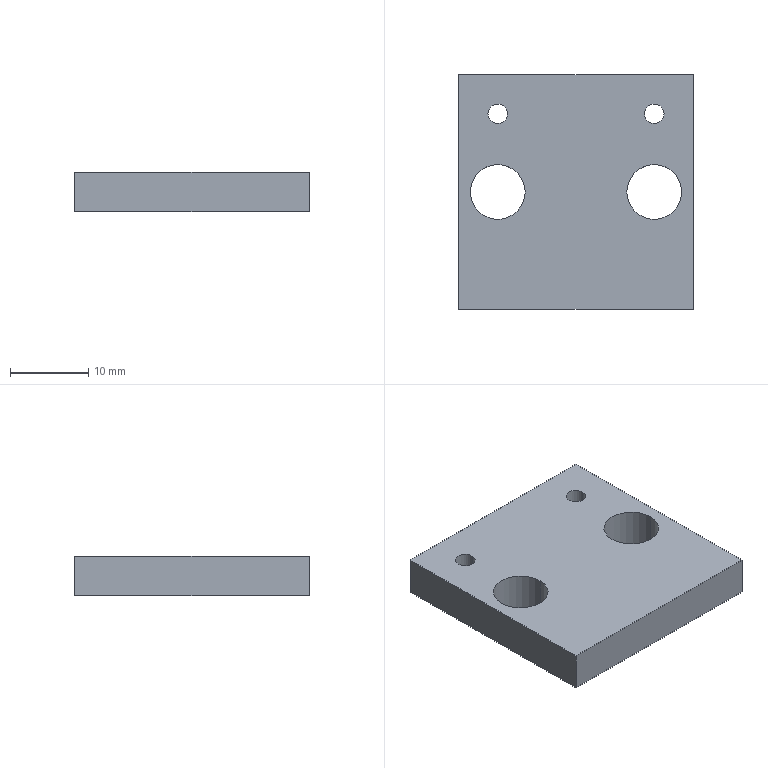Part | SolidWorks | features Extrusion 1, HoleWzd 1 | 1 solid | 14 faces | box 30 x 30 x 5 mm | volume 4066 mm3 | cylinder 8 | plane 6 | commonest cylinder face diameters 2.5 x4 7 x4
STEP:
#1=CARTESIAN_POINT('',(6.5,0.,0.));
#2=VERTEX_POINT('',#1);
#3=CARTESIAN_POINT('',(13.5,0.,0.));
#4=VERTEX_POINT('',#3);
#5=CARTESIAN_POINT('',(10.,0.,0.));
#6=DIRECTION('',(0.,0.,1.));
#7=DIRECTION('',(1.,0.,0.));
#8=AXIS2_PLACEMENT_3D('',#5,#6,#7);
#9=CIRCLE('',#8,3.5);
#10=EDGE_CURVE('',#2,#4,#9,.T.);
#11=ORIENTED_EDGE('',*,*,#10,.F.);
#12=CARTESIAN_POINT('',(6.5,0.,5.));
#13=VERTEX_POINT('',#12);
#14=CARTESIAN_POINT('',(6.5,0.,5.));
#15=DIRECTION('',(0.,0.,1.));
#16=VECTOR('',#15,1000.);
#17=LINE('',#14,#16);
#18=EDGE_CURVE('',#2,#13,#17,.T.);
#19=ORIENTED_EDGE('',*,*,#18,.T.);
#20=CARTESIAN_POINT('',(13.5,0.,5.));
#21=VERTEX_POINT('',#20);
#22=CARTESIAN_POINT('',(10.,0.,5.));
#23=DIRECTION('',(0.,0.,1.));
#24=DIRECTION('',(1.,0.,0.));
#25=AXIS2_PLACEMENT_3D('',#22,#23,#24);
#26=CIRCLE('',#25,3.5);
#27=EDGE_CURVE('',#13,#21,#26,.T.);
#28=ORIENTED_EDGE('',*,*,#27,.T.);
#29=CARTESIAN_POINT('',(13.5,0.,5.));
#30=DIRECTION('',(0.,0.,1.));
#31=VECTOR('',#30,1000.);
#32=LINE('',#29,#31);
#33=EDGE_CURVE('',#4,#21,#32,.T.);
#34=ORIENTED_EDGE('',*,*,#33,.F.);
#35=EDGE_LOOP('',(#11,#19,#28,#34));
#36=FACE_OUTER_BOUND('',#35,.T.);
#37=CARTESIAN_POINT('',(10.,0.,5.));
#38=DIRECTION('',(0.,0.,1.));
#39=DIRECTION('',(1.,0.,0.));
#40=AXIS2_PLACEMENT_3D('',#37,#38,#39);
#41=CYLINDRICAL_SURFACE('',#40,3.5);
#42=ADVANCED_FACE('',(#36),#41,.F.);
#43=CARTESIAN_POINT('',(-13.5,0.,0.));
#44=VERTEX_POINT('',#43);
#45=CARTESIAN_POINT('',(-6.5,0.,0.));
#46=VERTEX_POINT('',#45);
#47=CARTESIAN_POINT('',(-10.,0.,0.));
#48=DIRECTION('',(0.,0.,1.));
#49=DIRECTION('',(1.,0.,0.));
#50=AXIS2_PLACEMENT_3D('',#47,#48,#49);
#51=CIRCLE('',#50,3.5);
#52=EDGE_CURVE('',#44,#46,#51,.T.);
#53=ORIENTED_EDGE('',*,*,#52,.F.);
#54=CARTESIAN_POINT('',(-13.5,0.,5.));
#55=VERTEX_POINT('',#54);
#56=CARTESIAN_POINT('',(-13.5,0.,5.));
#57=DIRECTION('',(0.,0.,1.));
#58=VECTOR('',#57,1000.);
#59=LINE('',#56,#58);
#60=EDGE_CURVE('',#44,#55,#59,.T.);
#61=ORIENTED_EDGE('',*,*,#60,.T.);
#62=CARTESIAN_POINT('',(-6.5,0.,5.));
#63=VERTEX_POINT('',#62);
#64=CARTESIAN_POINT('',(-10.,0.,5.));
#65=DIRECTION('',(0.,0.,1.));
#66=DIRECTION('',(1.,0.,0.));
#67=AXIS2_PLACEMENT_3D('',#64,#65,#66);
#68=CIRCLE('',#67,3.5);
#69=EDGE_CURVE('',#55,#63,#68,.T.);
#70=ORIENTED_EDGE('',*,*,#69,.T.);
#71=CARTESIAN_POINT('',(-6.5,0.,5.));
#72=DIRECTION('',(0.,0.,1.));
#73=VECTOR('',#72,1000.);
#74=LINE('',#71,#73);
#75=EDGE_CURVE('',#46,#63,#74,.T.);
#76=ORIENTED_EDGE('',*,*,#75,.F.);
#77=EDGE_LOOP('',(#53,#61,#70,#76));
#78=FACE_OUTER_BOUND('',#77,.T.);
#79=CARTESIAN_POINT('',(-10.,0.,5.));
#80=DIRECTION('',(0.,0.,1.));
#81=DIRECTION('',(1.,0.,0.));
#82=AXIS2_PLACEMENT_3D('',#79,#80,#81);
#83=CYLINDRICAL_SURFACE('',#82,3.5);
#84=ADVANCED_FACE('',(#78),#83,.F.);
#85=CARTESIAN_POINT('',(8.75,10.,0.));
#86=VERTEX_POINT('',#85);
#87=CARTESIAN_POINT('',(11.25,10.,0.));
#88=VERTEX_POINT('',#87);
#89=CARTESIAN_POINT('',(10.,10.,0.));
#90=DIRECTION('',(0.,0.,1.));
#91=DIRECTION('',(-1.,0.,0.));
#92=AXIS2_PLACEMENT_3D('',#89,#90,#91);
#93=CIRCLE('',#92,1.25);
#94=EDGE_CURVE('',#86,#88,#93,.T.);
#95=ORIENTED_EDGE('',*,*,#94,.F.);
#96=CARTESIAN_POINT('',(8.75,10.,5.));
#97=VERTEX_POINT('',#96);
#98=CARTESIAN_POINT('',(8.75,10.,0.));
#99=DIRECTION('',(0.,0.,1.));
#100=VECTOR('',#99,1000.);
#101=LINE('',#98,#100);
#102=EDGE_CURVE('',#86,#97,#101,.T.);
#103=ORIENTED_EDGE('',*,*,#102,.T.);
#104=CARTESIAN_POINT('',(11.25,10.,5.));
#105=VERTEX_POINT('',#104);
#106=CARTESIAN_POINT('',(10.,10.,5.));
#107=DIRECTION('',(0.,0.,1.));
#108=DIRECTION('',(-1.,0.,0.));
#109=AXIS2_PLACEMENT_3D('',#106,#107,#108);
#110=CIRCLE('',#109,1.25);
#111=EDGE_CURVE('',#97,#105,#110,.T.);
#112=ORIENTED_EDGE('',*,*,#111,.T.);
#113=CARTESIAN_POINT('',(11.25,10.,0.));
#114=DIRECTION('',(0.,0.,1.));
#115=VECTOR('',#114,1000.);
#116=LINE('',#113,#115);
#117=EDGE_CURVE('',#88,#105,#116,.T.);
#118=ORIENTED_EDGE('',*,*,#117,.F.);
#119=EDGE_LOOP('',(#95,#103,#112,#118));
#120=FACE_OUTER_BOUND('',#119,.T.);
#121=CARTESIAN_POINT('',(10.,10.,0.));
#122=DIRECTION('',(0.,0.,1.));
#123=DIRECTION('',(1.,0.,0.));
#124=AXIS2_PLACEMENT_3D('',#121,#122,#123);
#125=CYLINDRICAL_SURFACE('',#124,1.25);
#126=ADVANCED_FACE('',(#120),#125,.F.);
#127=CARTESIAN_POINT('',(-11.25,10.,0.));
#128=VERTEX_POINT('',#127);
#129=CARTESIAN_POINT('',(-8.75,10.,0.));
#130=VERTEX_POINT('',#129);
#131=CARTESIAN_POINT('',(-10.,10.,0.));
#132=DIRECTION('',(0.,0.,1.));
#133=DIRECTION('',(-1.,0.,0.));
#134=AXIS2_PLACEMENT_3D('',#131,#132,#133);
#135=CIRCLE('',#134,1.25);
#136=EDGE_CURVE('',#128,#130,#135,.T.);
#137=ORIENTED_EDGE('',*,*,#136,.F.);
#138=CARTESIAN_POINT('',(-11.25,10.,5.));
#139=VERTEX_POINT('',#138);
#140=CARTESIAN_POINT('',(-11.25,10.,0.));
#141=DIRECTION('',(0.,0.,1.));
#142=VECTOR('',#141,1000.);
#143=LINE('',#140,#142);
#144=EDGE_CURVE('',#128,#139,#143,.T.);
#145=ORIENTED_EDGE('',*,*,#144,.T.);
#146=CARTESIAN_POINT('',(-8.75,10.,5.));
#147=VERTEX_POINT('',#146);
#148=CARTESIAN_POINT('',(-10.,10.,5.));
#149=DIRECTION('',(0.,0.,1.));
#150=DIRECTION('',(-1.,0.,0.));
#151=AXIS2_PLACEMENT_3D('',#148,#149,#150);
#152=CIRCLE('',#151,1.25);
#153=EDGE_CURVE('',#139,#147,#152,.T.);
#154=ORIENTED_EDGE('',*,*,#153,.T.);
#155=CARTESIAN_POINT('',(-8.75,10.,0.));
#156=DIRECTION('',(0.,0.,1.));
#157=VECTOR('',#156,1000.);
#158=LINE('',#155,#157);
#159=EDGE_CURVE('',#130,#147,#158,.T.);
#160=ORIENTED_EDGE('',*,*,#159,.F.);
#161=EDGE_LOOP('',(#137,#145,#154,#160));
#162=FACE_OUTER_BOUND('',#161,.T.);
#163=CARTESIAN_POINT('',(-10.,10.,0.));
#164=DIRECTION('',(0.,0.,1.));
#165=DIRECTION('',(1.,0.,0.));
#166=AXIS2_PLACEMENT_3D('',#163,#164,#165);
#167=CYLINDRICAL_SURFACE('',#166,1.25);
#168=ADVANCED_FACE('',(#162),#167,.F.);
#169=CARTESIAN_POINT('',(-15.,15.,5.));
#170=VERTEX_POINT('',#169);
#171=CARTESIAN_POINT('',(-15.,-15.,5.));
#172=VERTEX_POINT('',#171);
#173=CARTESIAN_POINT('',(-15.,15.,5.));
#174=DIRECTION('',(0.,-1.,0.));
#175=VECTOR('',#174,1000.);
#176=LINE('',#173,#175);
#177=EDGE_CURVE('',#170,#172,#176,.T.);
#178=ORIENTED_EDGE('',*,*,#177,.F.);
#179=CARTESIAN_POINT('',(-15.,15.,0.));
#180=VERTEX_POINT('',#179);
#181=CARTESIAN_POINT('',(-15.,15.,0.));
#182=DIRECTION('',(0.,0.,1.));
#183=VECTOR('',#182,1000.);
#184=LINE('',#181,#183);
#185=EDGE_CURVE('',#180,#170,#184,.T.);
#186=ORIENTED_EDGE('',*,*,#185,.F.);
#187=CARTESIAN_POINT('',(-15.,-15.,0.));
#188=VERTEX_POINT('',#187);
#189=CARTESIAN_POINT('',(-15.,15.,0.));
#190=DIRECTION('',(0.,-1.,0.));
#191=VECTOR('',#190,1000.);
#192=LINE('',#189,#191);
#193=EDGE_CURVE('',#180,#188,#192,.T.);
#194=ORIENTED_EDGE('',*,*,#193,.T.);
#195=CARTESIAN_POINT('',(-15.,-15.,0.));
#196=DIRECTION('',(0.,0.,1.));
#197=VECTOR('',#196,1000.);
#198=LINE('',#195,#197);
#199=EDGE_CURVE('',#188,#172,#198,.T.);
#200=ORIENTED_EDGE('',*,*,#199,.T.);
#201=EDGE_LOOP('',(#178,#186,#194,#200));
#202=FACE_OUTER_BOUND('',#201,.T.);
#203=CARTESIAN_POINT('',(-15.,15.,0.));
#204=DIRECTION('',(-1.,0.,0.));
#205=DIRECTION('',(0.,-1.,0.));
#206=AXIS2_PLACEMENT_3D('',#203,#204,#205);
#207=PLANE('',#206);
#208=ADVANCED_FACE('',(#202),#207,.T.);
#209=CARTESIAN_POINT('',(15.,15.,5.));
#210=VERTEX_POINT('',#209);
#211=CARTESIAN_POINT('',(15.,15.,5.));
#212=DIRECTION('',(-1.,0.,0.));
#213=VECTOR('',#212,1000.);
#214=LINE('',#211,#213);
#215=EDGE_CURVE('',#210,#170,#214,.T.);
#216=ORIENTED_EDGE('',*,*,#215,.F.);
#217=CARTESIAN_POINT('',(15.,15.,0.));
#218=VERTEX_POINT('',#217);
#219=CARTESIAN_POINT('',(15.,15.,0.));
#220=DIRECTION('',(0.,0.,1.));
#221=VECTOR('',#220,1000.);
#222=LINE('',#219,#221);
#223=EDGE_CURVE('',#218,#210,#222,.T.);
#224=ORIENTED_EDGE('',*,*,#223,.F.);
#225=CARTESIAN_POINT('',(15.,15.,0.));
#226=DIRECTION('',(-1.,0.,0.));
#227=VECTOR('',#226,1000.);
#228=LINE('',#225,#227);
#229=EDGE_CURVE('',#218,#180,#228,.T.);
#230=ORIENTED_EDGE('',*,*,#229,.T.);
#231=ORIENTED_EDGE('',*,*,#185,.T.);
#232=EDGE_LOOP('',(#216,#224,#230,#231));
#233=FACE_OUTER_BOUND('',#232,.T.);
#234=CARTESIAN_POINT('',(15.,15.,0.));
#235=DIRECTION('',(0.,1.,0.));
#236=DIRECTION('',(-1.,0.,0.));
#237=AXIS2_PLACEMENT_3D('',#234,#235,#236);
#238=PLANE('',#237);
#239=ADVANCED_FACE('',(#233),#238,.T.);
#240=CARTESIAN_POINT('',(15.,-15.,5.));
#241=VERTEX_POINT('',#240);
#242=CARTESIAN_POINT('',(15.,-15.,5.));
#243=DIRECTION('',(0.,1.,0.));
#244=VECTOR('',#243,1000.);
#245=LINE('',#242,#244);
#246=EDGE_CURVE('',#241,#210,#245,.T.);
#247=ORIENTED_EDGE('',*,*,#246,.F.);
#248=CARTESIAN_POINT('',(15.,-15.,0.));
#249=VERTEX_POINT('',#248);
#250=CARTESIAN_POINT('',(15.,-15.,0.));
#251=DIRECTION('',(0.,0.,1.));
#252=VECTOR('',#251,1000.);
#253=LINE('',#250,#252);
#254=EDGE_CURVE('',#249,#241,#253,.T.);
#255=ORIENTED_EDGE('',*,*,#254,.F.);
#256=CARTESIAN_POINT('',(15.,-15.,0.));
#257=DIRECTION('',(0.,1.,0.));
#258=VECTOR('',#257,1000.);
#259=LINE('',#256,#258);
#260=EDGE_CURVE('',#249,#218,#259,.T.);
#261=ORIENTED_EDGE('',*,*,#260,.T.);
#262=ORIENTED_EDGE('',*,*,#223,.T.);
#263=EDGE_LOOP('',(#247,#255,#261,#262));
#264=FACE_OUTER_BOUND('',#263,.T.);
#265=CARTESIAN_POINT('',(15.,-15.,0.));
#266=DIRECTION('',(1.,0.,0.));
#267=DIRECTION('',(0.,1.,0.));
#268=AXIS2_PLACEMENT_3D('',#265,#266,#267);
#269=PLANE('',#268);
#270=ADVANCED_FACE('',(#264),#269,.T.);
#271=CARTESIAN_POINT('',(-15.,-15.,5.));
#272=DIRECTION('',(1.,0.,0.));
#273=VECTOR('',#272,1000.);
#274=LINE('',#271,#273);
#275=EDGE_CURVE('',#172,#241,#274,.T.);
#276=ORIENTED_EDGE('',*,*,#275,.F.);
#277=ORIENTED_EDGE('',*,*,#199,.F.);
#278=CARTESIAN_POINT('',(-15.,-15.,0.));
#279=DIRECTION('',(1.,0.,0.));
#280=VECTOR('',#279,1000.);
#281=LINE('',#278,#280);
#282=EDGE_CURVE('',#188,#249,#281,.T.);
#283=ORIENTED_EDGE('',*,*,#282,.T.);
#284=ORIENTED_EDGE('',*,*,#254,.T.);
#285=EDGE_LOOP('',(#276,#277,#283,#284));
#286=FACE_OUTER_BOUND('',#285,.T.);
#287=CARTESIAN_POINT('',(-15.,-15.,0.));
#288=DIRECTION('',(0.,-1.,0.));
#289=DIRECTION('',(1.,0.,0.));
#290=AXIS2_PLACEMENT_3D('',#287,#288,#289);
#291=PLANE('',#290);
#292=ADVANCED_FACE('',(#286),#291,.T.);
#293=CARTESIAN_POINT('',(10.,0.,0.));
#294=DIRECTION('',(0.,0.,1.));
#295=DIRECTION('',(1.,0.,0.));
#296=AXIS2_PLACEMENT_3D('',#293,#294,#295);
#297=CIRCLE('',#296,3.5);
#298=EDGE_CURVE('',#4,#2,#297,.T.);
#299=ORIENTED_EDGE('',*,*,#298,.T.);
#300=ORIENTED_EDGE('',*,*,#10,.T.);
#301=EDGE_LOOP('',(#299,#300));
#302=FACE_BOUND('',#301,.T.);
#303=CARTESIAN_POINT('',(-10.,0.,0.));
#304=DIRECTION('',(0.,0.,1.));
#305=DIRECTION('',(1.,0.,0.));
#306=AXIS2_PLACEMENT_3D('',#303,#304,#305);
#307=CIRCLE('',#306,3.5);
#308=EDGE_CURVE('',#46,#44,#307,.T.);
#309=ORIENTED_EDGE('',*,*,#308,.T.);
#310=ORIENTED_EDGE('',*,*,#52,.T.);
#311=EDGE_LOOP('',(#309,#310));
#312=FACE_BOUND('',#311,.T.);
#313=CARTESIAN_POINT('',(10.,10.,0.));
#314=DIRECTION('',(0.,0.,1.));
#315=DIRECTION('',(-1.,0.,0.));
#316=AXIS2_PLACEMENT_3D('',#313,#314,#315);
#317=CIRCLE('',#316,1.25);
#318=EDGE_CURVE('',#88,#86,#317,.T.);
#319=ORIENTED_EDGE('',*,*,#318,.T.);
#320=ORIENTED_EDGE('',*,*,#94,.T.);
#321=EDGE_LOOP('',(#319,#320));
#322=FACE_BOUND('',#321,.T.);
#323=CARTESIAN_POINT('',(-10.,10.,0.));
#324=DIRECTION('',(0.,0.,1.));
#325=DIRECTION('',(-1.,0.,0.));
#326=AXIS2_PLACEMENT_3D('',#323,#324,#325);
#327=CIRCLE('',#326,1.25);
#328=EDGE_CURVE('',#130,#128,#327,.T.);
#329=ORIENTED_EDGE('',*,*,#328,.T.);
#330=ORIENTED_EDGE('',*,*,#136,.T.);
#331=EDGE_LOOP('',(#329,#330));
#332=FACE_BOUND('',#331,.T.);
#333=ORIENTED_EDGE('',*,*,#193,.F.);
#334=ORIENTED_EDGE('',*,*,#229,.F.);
#335=ORIENTED_EDGE('',*,*,#260,.F.);
#336=ORIENTED_EDGE('',*,*,#282,.F.);
#337=EDGE_LOOP('',(#333,#334,#335,#336));
#338=FACE_OUTER_BOUND('',#337,.T.);
#339=CARTESIAN_POINT('',(0.,0.,0.));
#340=DIRECTION('',(0.,0.,1.));
#341=DIRECTION('',(1.,0.,0.));
#342=AXIS2_PLACEMENT_3D('',#339,#340,#341);
#343=PLANE('',#342);
#344=ADVANCED_FACE('',(#302,#312,#322,#332,#338),#343,.F.);
#345=CARTESIAN_POINT('',(10.,0.,5.));
#346=DIRECTION('',(0.,0.,1.));
#347=DIRECTION('',(1.,0.,0.));
#348=AXIS2_PLACEMENT_3D('',#345,#346,#347);
#349=CIRCLE('',#348,3.5);
#350=EDGE_CURVE('',#21,#13,#349,.T.);
#351=ORIENTED_EDGE('',*,*,#350,.F.);
#352=ORIENTED_EDGE('',*,*,#27,.F.);
#353=EDGE_LOOP('',(#351,#352));
#354=FACE_BOUND('',#353,.T.);
#355=CARTESIAN_POINT('',(-10.,0.,5.));
#356=DIRECTION('',(0.,0.,1.));
#357=DIRECTION('',(1.,0.,0.));
#358=AXIS2_PLACEMENT_3D('',#355,#356,#357);
#359=CIRCLE('',#358,3.5);
#360=EDGE_CURVE('',#63,#55,#359,.T.);
#361=ORIENTED_EDGE('',*,*,#360,.F.);
#362=ORIENTED_EDGE('',*,*,#69,.F.);
#363=EDGE_LOOP('',(#361,#362));
#364=FACE_BOUND('',#363,.T.);
#365=CARTESIAN_POINT('',(10.,10.,5.));
#366=DIRECTION('',(0.,0.,1.));
#367=DIRECTION('',(-1.,0.,0.));
#368=AXIS2_PLACEMENT_3D('',#365,#366,#367);
#369=CIRCLE('',#368,1.25);
#370=EDGE_CURVE('',#105,#97,#369,.T.);
#371=ORIENTED_EDGE('',*,*,#370,.F.);
#372=ORIENTED_EDGE('',*,*,#111,.F.);
#373=EDGE_LOOP('',(#371,#372));
#374=FACE_BOUND('',#373,.T.);
#375=CARTESIAN_POINT('',(-10.,10.,5.));
#376=DIRECTION('',(0.,0.,1.));
#377=DIRECTION('',(-1.,0.,0.));
#378=AXIS2_PLACEMENT_3D('',#375,#376,#377);
#379=CIRCLE('',#378,1.25);
#380=EDGE_CURVE('',#147,#139,#379,.T.);
#381=ORIENTED_EDGE('',*,*,#380,.F.);
#382=ORIENTED_EDGE('',*,*,#153,.F.);
#383=EDGE_LOOP('',(#381,#382));
#384=FACE_BOUND('',#383,.T.);
#385=ORIENTED_EDGE('',*,*,#177,.T.);
#386=ORIENTED_EDGE('',*,*,#275,.T.);
#387=ORIENTED_EDGE('',*,*,#246,.T.);
#388=ORIENTED_EDGE('',*,*,#215,.T.);
#389=EDGE_LOOP('',(#385,#386,#387,#388));
#390=FACE_OUTER_BOUND('',#389,.T.);
#391=CARTESIAN_POINT('',(0.,0.,5.));
#392=DIRECTION('',(0.,0.,1.));
#393=DIRECTION('',(1.,0.,0.));
#394=AXIS2_PLACEMENT_3D('',#391,#392,#393);
#395=PLANE('',#394);
#396=ADVANCED_FACE('',(#354,#364,#374,#384,#390),#395,.T.);
#397=ORIENTED_EDGE('',*,*,#144,.F.);
#398=ORIENTED_EDGE('',*,*,#328,.F.);
#399=ORIENTED_EDGE('',*,*,#159,.T.);
#400=ORIENTED_EDGE('',*,*,#380,.T.);
#401=EDGE_LOOP('',(#397,#398,#399,#400));
#402=FACE_OUTER_BOUND('',#401,.T.);
#403=CARTESIAN_POINT('',(-10.,10.,0.));
#404=DIRECTION('',(0.,0.,1.));
#405=DIRECTION('',(1.,0.,0.));
#406=AXIS2_PLACEMENT_3D('',#403,#404,#405);
#407=CYLINDRICAL_SURFACE('',#406,1.25);
#408=ADVANCED_FACE('',(#402),#407,.F.);
#409=ORIENTED_EDGE('',*,*,#102,.F.);
#410=ORIENTED_EDGE('',*,*,#318,.F.);
#411=ORIENTED_EDGE('',*,*,#117,.T.);
#412=ORIENTED_EDGE('',*,*,#370,.T.);
#413=EDGE_LOOP('',(#409,#410,#411,#412));
#414=FACE_OUTER_BOUND('',#413,.T.);
#415=CARTESIAN_POINT('',(10.,10.,0.));
#416=DIRECTION('',(0.,0.,1.));
#417=DIRECTION('',(1.,0.,0.));
#418=AXIS2_PLACEMENT_3D('',#415,#416,#417);
#419=CYLINDRICAL_SURFACE('',#418,1.25);
#420=ADVANCED_FACE('',(#414),#419,.F.);
#421=ORIENTED_EDGE('',*,*,#60,.F.);
#422=ORIENTED_EDGE('',*,*,#308,.F.);
#423=ORIENTED_EDGE('',*,*,#75,.T.);
#424=ORIENTED_EDGE('',*,*,#360,.T.);
#425=EDGE_LOOP('',(#421,#422,#423,#424));
#426=FACE_OUTER_BOUND('',#425,.T.);
#427=CARTESIAN_POINT('',(-10.,0.,5.));
#428=DIRECTION('',(0.,0.,1.));
#429=DIRECTION('',(1.,0.,0.));
#430=AXIS2_PLACEMENT_3D('',#427,#428,#429);
#431=CYLINDRICAL_SURFACE('',#430,3.5);
#432=ADVANCED_FACE('',(#426),#431,.F.);
#433=ORIENTED_EDGE('',*,*,#18,.F.);
#434=ORIENTED_EDGE('',*,*,#298,.F.);
#435=ORIENTED_EDGE('',*,*,#33,.T.);
#436=ORIENTED_EDGE('',*,*,#350,.T.);
#437=EDGE_LOOP('',(#433,#434,#435,#436));
#438=FACE_OUTER_BOUND('',#437,.T.);
#439=CARTESIAN_POINT('',(10.,0.,5.));
#440=DIRECTION('',(0.,0.,1.));
#441=DIRECTION('',(1.,0.,0.));
#442=AXIS2_PLACEMENT_3D('',#439,#440,#441);
#443=CYLINDRICAL_SURFACE('',#442,3.5);
#444=ADVANCED_FACE('',(#438),#443,.F.);
#445=CLOSED_SHELL('',(#42,#84,#126,#168,#208,#239,#270,#292,#344,#396,#408,#420,#432,#444));
#446=MANIFOLD_SOLID_BREP('',#445);
#447=CARTESIAN_POINT('',(0.,0.,0.));
#448=DIRECTION('',(0.,0.,1.));
#449=DIRECTION('',(1.,0.,0.));
#450=AXIS2_PLACEMENT_3D('',#447,#448,#449);
#451=(LENGTH_UNIT()NAMED_UNIT(*)SI_UNIT(.MILLI.,.METRE.));
#452=UNCERTAINTY_MEASURE_WITH_UNIT(LENGTH_MEASURE(0.00001),#451,'','');
#453=(NAMED_UNIT(*)PLANE_ANGLE_UNIT()SI_UNIT($,.RADIAN.));
#454=(NAMED_UNIT(*)SI_UNIT($,.STERADIAN.)SOLID_ANGLE_UNIT());
#455=(GEOMETRIC_REPRESENTATION_CONTEXT(3)GLOBAL_UNCERTAINTY_ASSIGNED_CONTEXT((#452))GLOBAL_UNIT_ASSIGNED_CONTEXT((#451,#453,#454))REPRESENTATION_CONTEXT('',''));
#456=ADVANCED_BREP_SHAPE_REPRESENTATION('',(#446,#450),#455);